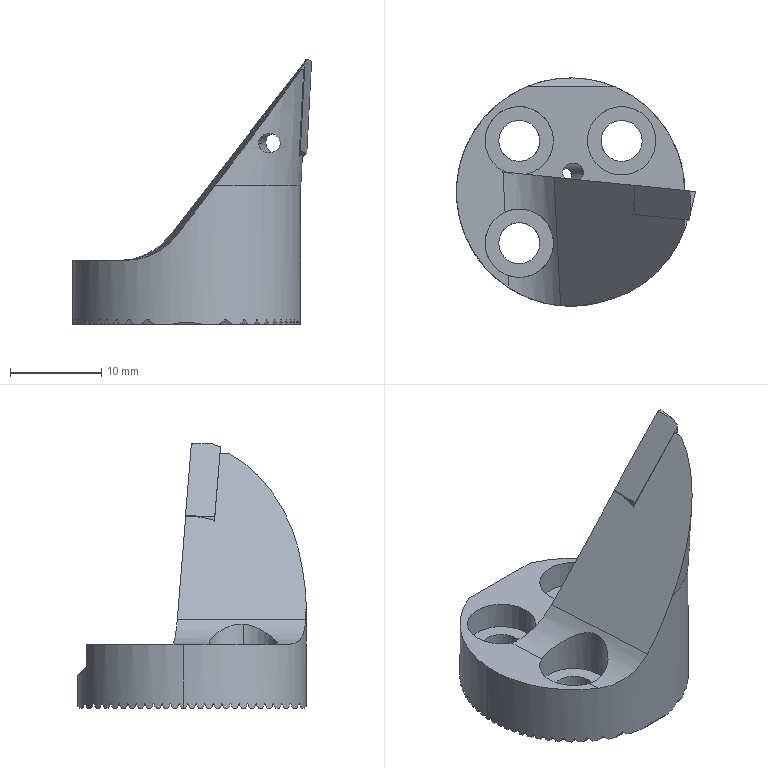NC program | Mastercam | posted with a generic post
Lines 3016 to 4664 of 4664, first 1474 of 1649 lines:
(6 FEM |TOOL - 1|DIA. OFF. - 1|LEN. - 1|TOOL DIA. - 6.)
N6096 T1 M6
N6098 G0 G54 G90 X10.395 Y-5.569 C85.98 B-29.925 S3500 M3
N6100 G43 H1 Z61.524
N6102 Z12.524
N6104 G1 Z11.324 F2000.
N6106 G41 D1 X8.435 Y-5.169 F400.
N6108 X2.979 Y-4.057
N6110 X2.948 Y-4.561
N6112 X8.336 Y-5.659
N6114 G40 X10.295 Y-6.059
N6116 X10.395 Y-5.569
N6118 Z11.124 F2000.
N6120 G41 D1 X8.435 Y-5.169 F400.
N6122 X2.979 Y-4.057
N6124 X2.948 Y-4.561
N6126 X8.336 Y-5.659
N6128 G40 X10.295 Y-6.059
N6130 X10.395 Y-5.569
N6132 Z10.924 F2000.
N6134 G41 D1 X8.435 Y-5.169 F400.
N6136 X2.979 Y-4.057
N6138 X2.948 Y-4.561
N6140 X8.336 Y-5.659
N6142 G40 X10.295 Y-6.059
N6144 X10.395 Y-5.569
N6146 Z10.724 F2000.
N6148 G41 D1 X8.435 Y-5.169 F400.
N6150 X2.979 Y-4.057
N6152 X2.948 Y-4.561
N6154 X8.336 Y-5.659
N6156 G40 X10.295 Y-6.059
N6158 X10.395 Y-5.569
N6160 Z10.524 F2000.
N6162 G41 D1 X8.435 Y-5.169 F400.
N6164 X2.979 Y-4.057
N6166 X2.948 Y-4.561
N6168 X8.336 Y-5.659
N6170 G40 X10.295 Y-6.059
N6172 X10.395 Y-5.569
N6174 Z10.324 F2000.
N6176 G41 D1 X8.435 Y-5.169 F400.
N6178 X2.979 Y-4.057
N6180 X2.948 Y-4.561
N6182 X8.336 Y-5.659
N6184 G40 X10.295 Y-6.059
N6186 X10.395 Y-5.569
N6188 Z10.124 F2000.
N6190 G41 D1 X8.435 Y-5.169 F400.
N6192 X2.979 Y-4.057
N6194 X2.948 Y-4.561
N6196 X8.336 Y-5.659
N6198 G40 X10.295 Y-6.059
N6200 X10.395 Y-5.569
N6202 Z9.924 F2000.
N6204 G41 D1 X8.435 Y-5.169 F400.
N6206 X2.979 Y-4.057
N6208 X2.948 Y-4.561
N6210 X8.336 Y-5.659
N6212 G40 X10.295 Y-6.059
N6214 G0 Z61.524
N6216 M5
N6218 G0 G28 G91 Z0.
N6220 G28 C0. B0.
N6222 M01
N6224 G0 G17 G40 G80 G90 G94 G98
N6226 G0 G28 G91 Z0.
(2 DR |TOOL - 2|DIA. OFF. - 2|LEN. - 2|TOOL DIA. - 2.)
N6228 T2 M6
N6230 G0 G54 G90 X3.096 Y-2.135 C85.98 B-29.925 S150 M3
N6232 G43 H2 Z60.924
N6234 G83 G98 Z2.424 R11.924 Q2. F10.
N6236 G80
N6238 M5
N6240 G0 G28 G91 Z0.
N6242 G28 C0. B0.
N6244 M01
N6246 G0 G17 G40 G80 G90 G94 G98
N6248 G0 G28 G91 Z0.
(12 FEMR |TOOL - 4|DIA. OFF. - 4|LEN. - 4|TOOL DIA. - 12.)
N6250 T4 M6
N6252 G0 G54 G90 X14.729 Y22.915 C6. B-90. S3500 M3
N6254 G43 H4 Z61.514
N6256 Z3.514
N6258 G1 Z1.764 F2000.
N6260 X14.032 Y21.345 Z1.613 F2500.
N6262 G3 X13.8 Y20.25 Z1.514 I2.468 J-1.095
N6264 G1 Y19.651
N6266 Y19.47
N6268 G2 X14.97 Y18.269 I-45.936 J-45.932
N6270 X16.838 Y14.761 I-6.985 J-5.971
N6272 X17.407 Y11.333 I-15.59 J-4.35
N6274 X17.54 Y6.9 I-73.653 J-4.433
N6276 G1 Y6.592
N6278 G2 X17.549 Y2.503 I-899.541 J-4.089
N6280 G1 Y2.175
N6282 Y1.775
N6284 X17.54 Y-12.63
N6286 G2 X16.333 Y-15.954 I-6.352 J.425
N6288 X13.8 Y-18.183 I-6.198 J4.49
N6290 G1 Y-18.582
N6292 Y-18.981
N6294 G3 X16.031 Y-21.64 Z1.764 I2.7
N6296 X16.5 Y-21.681 I.469 J2.659 F9500.
N6298 X19.2 Y-18.981 J2.7
N6300 G1 Y19.725
N6302 G3 X16.5 Y22.425 I-2.7
N6304 X16.031 Y22.384 J-2.7
N6306 X13.8 Y19.725 Z1.514 I.469 J-2.659 F2500.
N6308 G1 Y19.127
N6310 Y18.921
N6312 X14.784 Y17.652
N6314 G2 X16.575 Y13.738 I-9.517 J-6.721
N6316 X17.136 Y10.072 I-19.858 J-4.918
N6318 X17.286 Y5.071 I-83.135 J-5.001
N6320 X17.287 Y4.942 I-83.285
N6322 X17.299 Y.199 I-906.994 J-4.743
N6324 G1 Y-.279
N6326 Y-.679
N6328 X17.297 Y-10.765
N6330 G2 X16.016 Y-14.965 I-7.969 J.136
N6332 X14.326 Y-17.063 I-9.858 J6.212
N6334 G3 X13.905 Y-17.528 I1.14 J-1.455
N6336 X13.8 Y-17.781 I1.048 J-.584
N6338 G1 X14.729 Y-17.96 Z1.576
N6340 G3 X15.651 Y-18.048 Z1.638 I.922 J4.789
N6342 X17.5 Y-17.684 Z1.764 J4.877
N6344 X20.528 Y-13.171 I-1.849 J4.513 F9500.
N6346 X20.516 Y-12.826 I-4.877
N6348 G1 X18.722 Y12.481
N6350 G3 X17.618 Y16.38 I-9.929 J-.704
N6352 G1 X15.156 Y21.1
N6354 X14.729 Y21.919 Z1.702 F2500.
N6356 X14.032 Y20.35 Z1.588
N6358 G3 X13.8 Y19.254 Z1.514 I2.468 J-1.096
N6360 G1 Y18.656
N6362 Y18.445
N6364 X14.667 Y17.103
N6366 G2 X16.375 Y12.756 I-12.15 J-7.284
N6368 X16.922 Y8.354 I-26.107 J-5.48
N6370 X17.043 Y2.631 I-134.973 J-5.723
N6372 G1 X17.042 Y2.11
N6374 G2 X17.047 Y.103 I-910.2 J-3.046
N6376 G1 X17.048 Y-.297
N6378 X17.037 Y-9.694
N6380 G2 X15.43 Y-14.831 I-10.263 J.39
N6382 X14.377 Y-16.348 I-14.569 J8.986
N6384 G1 X14.075 Y-16.691
N6386 G3 X13.8 Y-17.242 I.9 J-.793
N6388 G1 X14.729 Y-17.37 Z1.576
N6390 G3 X15.096 Y-17.395 Z1.6 I.367 J2.675
N6392 X17.232 Y-16.346 Z1.764 J2.7
N6394 X17.791 Y-14.856 I-2.136 J1.651 F9500.
N6396 G1 X19.892 Y20.223
N6398 G3 X19.897 Y20.384 I-2.695 J.161
N6400 X17.197 Y23.084 I-2.7
N6402 X15.24 Y22.245 J-2.7
N6404 X14.729 Y21.48 Z1.702 I1.957 J-1.861 F2500.
N6406 G1 X14.032 Y19.91 Z1.588
N6408 G3 X13.8 Y18.815 Z1.514 I2.468 J-1.095
N6410 G1 Y18.216
N6412 Y17.994
N6414 X14.589 Y16.547
N6416 G2 X16.285 Y11.268 I-15.796 J-7.987
N6418 X16.704 Y6.65 I-36.902 J-5.679
N6420 X16.798 Y-.081 I-239.814 J-6.731
N6422 X16.797 Y-1.122 I-239.908
N6424 G1 Y-1.523
N6426 G2 X16.8 Y-3.681 I-906.97 J-2.158
N6428 X16.787 Y-8.476 I-906.973
N6430 X15.077 Y-14.518 I-12.293 J.216
N6432 X14.239 Y-15.883 I-26.241 J15.167
N6434 G1 X14.033 Y-16.164
N6436 G3 X13.8 Y-16.875 I.967 J-.711
N6438 X16.031 Y-19.534 Z1.764 I2.7
N6440 X16.5 Y-19.575 I.469 J2.659 F9500.
N6442 X19.2 Y-16.875 J2.7
N6444 G1 Y18.386
N6446 G3 X16.5 Y21.086 I-2.7
N6448 X16.031 Y21.045 J-2.7
N6450 X13.8 Y18.386 Z1.514 I.469 J-2.659 F2500.
N6452 G1 Y17.787
N6454 Y17.549
N6456 X14.628 Y15.739
N6458 G2 X16.102 Y10.224 I-19.714 J-8.227
N6460 X16.482 Y4.878 I-48.834 J-6.152
N6462 X16.552 Y-3.377 I-483.428 J-8.255
N6464 X16.549 Y-5.233 I-483.498
N6466 G1 Y-5.633
N6468 G2 X16.552 Y-6.149 I-39.576 J-.516
N6470 X16.488 Y-8.413 I-39.579
N6472 X14.888 Y-14.011 I-14.099 J1.
N6474 X13.984 Y-15.667 I-35.691 J18.427
N6476 G3 X13.8 Y-16.305 I1.016 J-.638
N6478 X16.031 Y-18.964 Z1.764 I2.7
N6480 X16.5 Y-19.005 I.469 J2.659 F9500.
N6482 X19.2 Y-16.305 J2.7
N6484 G1 Y17.963
N6486 G3 X16.5 Y20.663 I-2.7
N6488 X16.031 Y20.622 J-2.7
N6490 X13.8 Y17.963 Z1.514 I.469 J-2.659 F2500.
N6492 G1 Y17.365
N6494 Y17.099
N6496 X14.625 Y14.949
N6498 G2 X15.966 Y8.715 I-24.973 J-8.635
N6500 X16.259 Y2.691 I-71.608 J-6.502
N6502 X16.294 Y-2.883 I-438.719 J-5.574
N6504 X16.277 Y-6.733 I-438.754
N6506 X14.619 Y-13.723 I-16.545 J.233
N6508 G3 X14.142 Y-14.741 I131.524 J-62.248
N6510 G1 X13.926 Y-15.188
N6512 G3 X13.8 Y-15.724 I1.076 J-.536
N6514 G1 Y-16.123
N6516 G3 X16.031 Y-18.782 Z1.764 I2.7
N6518 X16.5 Y-18.823 I.469 J2.659 F9500.
N6520 X19.2 Y-16.123 J2.7
N6522 G1 Y17.537
N6524 G3 X16.5 Y20.237 I-2.7
N6526 X16.031 Y20.196 J-2.7
N6528 X13.8 Y17.537 Z1.514 I.469 J-2.659 F2500.
N6530 G1 Y16.938
N6532 Y16.634
N6534 X14.59 Y14.166
N6536 G2 X15.764 Y7.67 I-30.935 J-8.945
N6538 X16.016 Y1.314 I-88.563 J-6.705
N6540 X16.041 Y-2.954 I-361.608 J-4.268
N6542 X16.032 Y-5.648 I-361.633
N6544 X15.571 Y-9.827 I-20.824 J.181
N6546 X14.278 Y-13.684 I-21.736 J5.14
N6548 G3 X13.888 Y-14.663 I18.448 J-7.926
N6550 X13.8 Y-15.114 I1.112 J-.451
N6552 G1 Y-15.513
N6554 G3 X16.031 Y-18.172 Z1.764 I2.7
N6556 X16.5 Y-18.213 I.469 J2.659 F9500.
N6558 X19.2 Y-15.513 J2.7
N6560 G1 Y17.097
N6562 G3 X16.5 Y19.797 I-2.7
N6564 X16.031 Y19.756 J-2.7
N6566 X13.8 Y17.097 Z1.514 I.469 J-2.659 F2500.
N6568 G1 Y16.499
N6570 G3 X13.789 Y16.322 I1.462 J-.177
N6572 X13.883 Y15.804 I1.473
N6574 X14.089 Y15.056 I143.834 J39.039
N6576 G2 X15.613 Y5.73 I-38.302 J-11.048
N6578 X15.785 Y-1.589 I-155.302 J-7.319
N6580 G1 Y-1.716
N6582 G2 X15.794 Y-2.931 I-85.343 J-1.215
N6584 X15.738 Y-6.002 I-85.352
N6586 X14.402 Y-12.5 I-21.07 J.949
N6588 G3 X13.852 Y-14.096 I31.212 J-11.635
N6590 X13.8 Y-14.447 I1.148 J-.351
N6592 G1 Y-14.846
N6594 G3 X16.031 Y-17.505 Z1.764 I2.7
N6596 X16.5 Y-17.546 I.469 J2.659 F9500.
N6598 X19.2 Y-14.846 J2.7
N6600 G1 Y16.636
N6602 G3 X16.5 Y19.336 I-2.7
N6604 X16.031 Y19.295 J-2.7
N6606 X13.8 Y16.636 Z1.514 I.469 J-2.659 F2500.
N6608 G1 Y16.037
N6610 G3 X13.793 Y15.857 I2.187 J-.18
N6612 X13.856 Y15.332 I2.194
N6614 X14.353 Y13.046 I139.853 J29.205
N6616 G2 X15.389 Y4.704 I-47.631 J-10.149
N6618 X15.527 Y-2.066 I-165.786 J-6.77
N6620 X15.503 Y-4.901 I-165.924
N6622 X14.207 Y-12.123 I-24.214 J.618
N6624 G3 X13.84 Y-13.357 I21.503 J-7.065
N6626 X13.795 Y-13.85 I2.68 J-.493
N6628 X13.8 Y-14.012 I2.725
N6630 G1 Y-14.412
N6632 G3 X16.031 Y-17.071 Z1.764 I2.7
N6634 X16.5 Y-17.112 I.469 J2.659 F9500.
N6636 X19.2 Y-14.412 J2.7
N6638 G1 Y16.154
N6640 G3 X16.5 Y18.854 I-2.7
N6642 X16.031 Y18.813 J-2.7
N6644 X13.8 Y16.154 Z1.514 I.469 J-2.659 F2500.
N6646 G1 Y15.555
N6648 G3 X13.795 Y15.356 I3.962 J-.199
N6650 X13.868 Y14.599 I3.967
N6652 X14.388 Y11.558 I128.842 J20.504
N6654 G2 X15.174 Y3.359 I-59.781 J-9.865
N6656 X15.268 Y-1.868 I-145.694 J-5.227
N6658 X15.25 Y-4.169 I-145.788
N6660 X14.153 Y-11.265 I-27.035 J.544
N6662 G3 X13.833 Y-12.478 I29.887 J-8.55
N6664 X13.791 Y-12.938 I2.486 J-.46
N6666 X13.8 Y-13.156 I2.528
N6668 G1 Y-13.555
N6670 Y-13.988
N6672 Y-13.998
N6674 Y-14.002
N6676 Y-14.212
N6678 Y-14.412
N6680 G3 X16.031 Y-17.071 Z1.764 I2.7
N6682 X16.5 Y-17.112 I.469 J2.659 F9500.
N6684 X19.2 Y-14.412 J2.7
N6686 G1 Y15.656
N6688 G3 X16.5 Y18.356 I-2.7
N6690 X16.031 Y18.315 J-2.7
N6692 X13.8 Y15.656 Z1.514 I.469 J-2.659 F2500.
N6694 G1 Y15.057
N6696 G3 X13.798 Y14.834 I10.86 J-.223
N6698 X13.934 Y13.115 I10.862
N6700 X14.261 Y10.786 I193.248 J25.883
N6702 G2 X14.955 Y1.87 I-75.072 J-10.337
N6704 X15.008 Y-1.441 I-103.205 J-3.311
N6706 X14.975 Y-4.057 I-103.258
N6708 X14.031 Y-10.578 I-30.027 J1.018
N6710 G3 X13.828 Y-11.453 I39.877 J-9.757
N6712 X13.79 Y-11.884 I2.422 J-.431
N6714 X13.8 Y-12.108 I2.46
N6716 G1 Y-12.508
N6718 Y-13.306
N6720 G3 X16.031 Y-15.965 Z1.764 I2.7
N6722 X16.5 Y-16.006 I.469 J2.659 F9500.
N6724 X19.2 Y-13.306 J2.7
N6726 G1 Y15.075
N6728 G3 X16.5 Y17.775 I-2.7
N6730 X16.031 Y17.734 J-2.7
N6732 X13.8 Y15.075 Z1.514 I.469 J-2.659 F2500.
N6734 G1 Y14.476
N6736 Y14.013
N6738 Y14.002
N6740 Y13.998
N6742 G3 X13.799 Y13.81 I17.867 J-.188
N6744 X13.972 Y11.33 I17.868
N6746 X14.105 Y10.152 I402.753 J44.877
N6748 G2 X14.739 Y-.314 I-96.738 J-11.111
N6750 X14.753 Y-1.498 I-50.081 J-1.184
N6752 X14.58 Y-5.654 I-50.095
N6754 X13.851 Y-10.113 I-37.302 J3.806
N6756 G3 X13.791 Y-10.675 I2.591 J-.562
N6758 X13.8 Y-10.891 I2.651
N6760 G1 Y-11.29
N6762 Y-12.088
N6764 G3 X16.031 Y-14.747 Z1.764 I2.7
N6766 X16.5 Y-14.788 I.469 J2.659 F9500.
N6768 X19.2 Y-12.088 J2.7
N6770 G1 Y14.147
N6772 G3 X16.5 Y16.847 I-2.7
N6774 X16.031 Y16.806 J-2.7
N6776 X13.8 Y14.147 Z1.514 I.469 J-2.659 F2500.
N6778 G1 Y14.08
N6780 Y13.998
N6782 Y13.569
N6784 Y13.15
N6786 Y12.751
N6788 G3 X13.797 Y12.368 I26.282 J-.383
N6790 X13.945 Y9.58 I26.285
N6792 X14.013 Y8.79 I806.017 J68.987
N6794 G2 X14.473 Y-1.324 I-110.84 J-10.114
N6796 X14.467 Y-2.527 I-111.3
N6798 X13.817 Y-8.84 I-37.065 J.629
N6800 G3 X13.791 Y-9.22 I2.763 J-.38
N6802 X13.8 Y-9.441 I2.789
N6804 G1 Y-9.84
N6806 Y-11.038
N6808 G3 X16.031 Y-13.697 Z1.764 I2.7
N6810 X16.5 Y-13.738 I.469 J2.659 F9500.
N6812 X19.2 Y-11.038 J2.7
N6814 G1 Y12.551
N6816 G3 X16.5 Y15.251 I-2.7
N6818 X16.031 Y15.21 J-2.7
N6820 X13.8 Y12.551 Z1.514 I.469 J-2.659 F2500.
N6822 G1 Y11.952
N6824 G3 X13.796 Y11.157 I89.637 J-.795
N6826 X13.83 Y8.678 I89.641
N6828 X14.031 Y5.13 I264.013 J13.129
N6830 G2 X14.206 Y-.867 I-102.867 J-5.997
N6832 X14.193 Y-2.466 I-103.042
N6834 X13.81 Y-7.07 I-39.426 J.959
N6836 G3 X13.792 Y-7.411 I3.189 J-.341
N6838 X13.8 Y-7.629 I3.207
N6840 G1 Y-8.028
N6842 Y-9.624
N6844 G3 X16.031 Y-12.283 Z1.764 I2.7
N6846 X16.5 Y-12.324 I.469 J2.659 F9500.
N6848 X19.2 Y-9.624 J2.7
N6850 G1 Y10.282
N6852 G3 X16.5 Y12.982 I-2.7
N6854 X16.031 Y12.941 J-2.7
N6856 X13.8 Y10.282 Z1.514 I.469 J-2.659 F2500.
N6858 G1 Y9.683
N6860 G3 X13.797 Y8.487 I264.088 J-1.196
N6862 X13.819 Y5.062 I264.091
N6864 X13.891 Y2.683 I526.245 J14.664
N6866 G2 X13.946 Y-.182 I-74.989 J-2.865
N6868 X13.88 Y-3.321 I-75.044
N6870 X13.8 Y-4.578 I-41.798 J2.036
N6872 G1 Y-4.977
N6874 Y-7.771
N6876 G3 X16.031 Y-10.43 Z1.764 I2.7
N6878 X16.5 Y-10.471 I.469 J2.659 F9500.
N6880 X19.2 Y-7.771 J2.7
N6882 G1 Y6.753
N6884 G3 X16.5 Y9.453 I-2.7
N6886 X16.031 Y9.412 J-2.7
N6888 X13.8 Y6.753 Z1.514 I.469 J-2.659 F2500.
N6890 G1 Y6.154
N6892 Y-5.021
N6894 G3 X14.032 Y-6.116 Z1.613 I2.7
N6896 G1 X14.729 Y-7.686 Z1.764
N6898 G0 Z61.514
N6900 X13.5 Y22.
N6902 Z52.214
N6904 Z3.214
N6906 G1 Z2.214 F2000.
N6908 G41 D4 Y14. F1000.
N6910 Y-14.
N6912 G40 Y-22.
N6914 G0 Z52.214
N6916 X13.1 Y22.
N6918 Z3.214
N6920 G1 Z2.214 F2000.
N6922 G41 D4 Y14. F1000.
N6924 Y-14.
N6926 G40 Y-22.
N6928 G0 Z52.214
N6930 Z62.563
N6932 X10.617 Y12.777
N6934 C0.
N6936 Z13.563
N6938 G1 Z12.113 F2000.
N6940 G41 D4 Y4.777 F1500.
N6942 Y-4.722
N6944 G40 Y-12.722
N6946 Z11.662 F2000.
N6948 G42 D4 Y-4.722 F1500.
N6950 Y4.777
N6952 G40 Y12.777
N6954 G0 Z62.563
N6956 B-45.
N6958 X-10.997 Y-12.722
N6960 Z62.405
N6962 Z13.405
N6964 G1 Z11.955 F2000.
N6966 G41 D4 Y-4.722 F1500.
N6968 Y4.777
N6970 G40 Y12.777
N6972 Z11.505 F2000.
N6974 G42 D4 Y4.777 F1500.
N6976 Y-4.722
N6978 G40 Y-12.722
N6980 G0 Z62.405
N6982 M5
N6984 G0 G28 G91 Z0.
N6986 G28 B0.
N6988 M01
N6990 G0 G17 G40 G80 G90 G94 G98
N6992 G0 G28 G91 Z0.
(3 FEMR |TOOL - 6|DIA. OFF. - 6|LEN. - 6|TOOL DIA. - 3.)
N6994 T6 M6
N6996 G0 G54 G90 X32.031 Y15.532 C6. B-90. S4500 M3
N6998 G43 H6 Z51.614
N7000 Z2.614
N7002 G1 Z1.422 F2000.
N7004 G41 D6 X31.11 Y15.141 F400.
N7006 X21.543 Y11.08
N7008 X20.313 Y10.119
N7010 X21.734 Y10.193
N7012 X31.173 Y14.2
N7014 G40 X32.094 Y14.591
N7016 X31.445 Y16.913
N7018 G41 D6 X30.524 Y16.522
N7020 X20.775 Y12.384
N7022 X16.033 Y8.679
N7024 X11.648 Y7.04
N7026 G3 X11.55 Y6.899 I.053 J-.141
N7028 X11.701 Y6.748 I.151
N7030 G1 X11.728 Y6.751
N7032 X11.753 Y6.758
N7034 X16.138 Y8.398
N7036 X22.076 Y8.709
N7038 X31.76 Y12.82
N7040 G40 X32.68 Y13.21
N7042 X32.031 Y15.532
N7044 Z1.231 F2000.
N7046 G41 D6 X31.11 Y15.141 F400.
N7048 X21.543 Y11.08
N7050 X20.313 Y10.119
N7052 X21.734 Y10.193
N7054 X31.173 Y14.2
N7056 G40 X32.094 Y14.591
N7058 X31.445 Y16.913
N7060 G41 D6 X30.524 Y16.522
N7062 X20.775 Y12.384
N7064 X16.033 Y8.679
N7066 X11.648 Y7.04
N7068 G3 X11.55 Y6.899 I.053 J-.141
N7070 X11.701 Y6.748 I.151
N7072 G1 X11.728 Y6.751
N7074 X11.753 Y6.758
N7076 X16.138 Y8.398
N7078 X22.076 Y8.709
N7080 X31.76 Y12.82
N7082 G40 X32.68 Y13.21
N7084 X32.031 Y15.532
N7086 Z1.039 F2000.
N7088 G41 D6 X31.11 Y15.141 F400.
N7090 X21.543 Y11.08
N7092 X20.313 Y10.119
N7094 X21.734 Y10.193
N7096 X31.173 Y14.2
N7098 G40 X32.094 Y14.591
N7100 X31.445 Y16.913
N7102 G41 D6 X30.524 Y16.522
N7104 X20.775 Y12.384
N7106 X16.033 Y8.679
N7108 X11.648 Y7.04
N7110 G3 X11.55 Y6.899 I.053 J-.141
N7112 X11.701 Y6.748 I.151
N7114 G1 X11.728 Y6.751
N7116 X11.753 Y6.758
N7118 X16.138 Y8.398
N7120 X22.076 Y8.709
N7122 X31.76 Y12.82
N7124 G40 X32.68 Y13.21
N7126 X32.031 Y15.532
N7128 Z.848 F2000.
N7130 G41 D6 X31.11 Y15.141 F400.
N7132 X21.543 Y11.08
N7134 X20.313 Y10.119
N7136 X21.734 Y10.193
N7138 X31.173 Y14.2
N7140 G40 X32.094 Y14.591
N7142 X31.445 Y16.913
N7144 G41 D6 X30.524 Y16.522
N7146 X20.775 Y12.384
N7148 X16.033 Y8.679
N7150 X11.648 Y7.04
N7152 G3 X11.55 Y6.899 I.053 J-.141
N7154 X11.701 Y6.748 I.151
N7156 G1 X11.728 Y6.751
N7158 X11.753 Y6.758
N7160 X16.138 Y8.398
N7162 X22.076 Y8.709
N7164 X31.76 Y12.82
N7166 G40 X32.68 Y13.21
N7168 X32.031 Y15.532
N7170 Z.656 F2000.
N7172 G41 D6 X31.11 Y15.141 F400.
N7174 X21.543 Y11.08
N7176 X20.313 Y10.119
N7178 X21.734 Y10.193
N7180 X31.173 Y14.2
N7182 G40 X32.094 Y14.591
N7184 X31.445 Y16.913
N7186 G41 D6 X30.524 Y16.522
N7188 X20.775 Y12.384
N7190 X16.033 Y8.679
N7192 X11.648 Y7.04
N7194 G3 X11.55 Y6.899 I.053 J-.141
N7196 X11.701 Y6.748 I.151
N7198 G1 X11.728 Y6.751
N7200 X11.753 Y6.758
N7202 X16.138 Y8.398
N7204 X22.076 Y8.709
N7206 X31.76 Y12.82
N7208 G40 X32.68 Y13.21
N7210 X32.031 Y15.532
N7212 Z.465 F2000.
N7214 G41 D6 X31.11 Y15.141 F400.
N7216 X21.543 Y11.08
N7218 X20.313 Y10.119
N7220 X21.734 Y10.193
N7222 X31.173 Y14.2
N7224 G40 X32.094 Y14.591
N7226 X31.445 Y16.913
N7228 G41 D6 X30.524 Y16.522
N7230 X20.775 Y12.384
N7232 X16.033 Y8.679
N7234 X11.648 Y7.04
N7236 G3 X11.55 Y6.899 I.053 J-.141
N7238 X11.701 Y6.748 I.151
N7240 G1 X11.728 Y6.751
N7242 X11.753 Y6.758
N7244 X16.138 Y8.398
N7246 X22.076 Y8.709
N7248 X31.76 Y12.82
N7250 G40 X32.68 Y13.21
N7252 X32.031 Y15.532
N7254 Z.273 F2000.
N7256 G41 D6 X31.11 Y15.141 F400.
N7258 X21.543 Y11.08
N7260 X20.313 Y10.119
N7262 X21.734 Y10.193
N7264 X31.173 Y14.2
N7266 G40 X32.094 Y14.591
N7268 X31.445 Y16.913
N7270 G41 D6 X30.524 Y16.522
N7272 X20.775 Y12.384
N7274 X16.033 Y8.679
N7276 X11.648 Y7.04
N7278 G3 X11.55 Y6.899 I.053 J-.141
N7280 X11.701 Y6.748 I.151
N7282 G1 X11.728 Y6.751
N7284 X11.753 Y6.758
N7286 X16.138 Y8.398
N7288 X22.076 Y8.709
N7290 X31.76 Y12.82
N7292 G40 X32.68 Y13.21
N7294 X32.031 Y15.532
N7296 Z.082 F2000.
N7298 G41 D6 X31.11 Y15.141 F400.
N7300 X21.543 Y11.08
N7302 X20.313 Y10.119
N7304 X21.734 Y10.193
N7306 X31.173 Y14.2
N7308 G40 X32.094 Y14.591
N7310 X31.445 Y16.913
N7312 G41 D6 X30.524 Y16.522
N7314 X20.775 Y12.384
N7316 X16.033 Y8.679
N7318 X11.648 Y7.04
N7320 G3 X11.55 Y6.899 I.053 J-.141
N7322 X11.701 Y6.748 I.151
N7324 G1 X11.728 Y6.751
N7326 X11.753 Y6.758
N7328 X16.138 Y8.398
N7330 X22.076 Y8.709
N7332 X31.76 Y12.82
N7334 G40 X32.68 Y13.21
N7336 X32.031 Y15.532
N7338 Z-.11 F2000.
N7340 G41 D6 X31.11 Y15.141 F400.
N7342 X21.543 Y11.08
N7344 X20.313 Y10.119
N7346 X21.734 Y10.193
N7348 X31.173 Y14.2
N7350 G40 X32.094 Y14.591
N7352 X31.445 Y16.913
N7354 G41 D6 X30.524 Y16.522
N7356 X20.775 Y12.384
N7358 X16.033 Y8.679
N7360 X11.648 Y7.04
N7362 G3 X11.55 Y6.899 I.053 J-.141
N7364 X11.701 Y6.748 I.151
N7366 G1 X11.728 Y6.751
N7368 X11.753 Y6.758
N7370 X16.138 Y8.398
N7372 X22.076 Y8.709
N7374 X31.76 Y12.82
N7376 G40 X32.68 Y13.21
N7378 X32.031 Y15.532
N7380 Z-.301 F2000.
N7382 G41 D6 X31.11 Y15.141 F400.
N7384 X21.543 Y11.08
N7386 X20.313 Y10.119
N7388 X21.734 Y10.193
N7390 X31.173 Y14.2
N7392 G40 X32.094 Y14.591
N7394 X31.445 Y16.913
N7396 G41 D6 X30.524 Y16.522
N7398 X20.775 Y12.384
N7400 X16.033 Y8.679
N7402 X11.648 Y7.04
N7404 G3 X11.55 Y6.899 I.053 J-.141
N7406 X11.701 Y6.748 I.151
N7408 G1 X11.728 Y6.751
N7410 X11.753 Y6.758
N7412 X16.138 Y8.398
N7414 X22.076 Y8.709
N7416 X31.76 Y12.82
N7418 G40 X32.68 Y13.21
N7420 X32.031 Y15.532
N7422 Z-.492 F2000.
N7424 G41 D6 X31.11 Y15.141 F400.
N7426 X21.543 Y11.08
N7428 X20.313 Y10.119
N7430 X21.734 Y10.193
N7432 X31.173 Y14.2
N7434 G40 X32.094 Y14.591
N7436 X31.445 Y16.913
N7438 G41 D6 X30.524 Y16.522
N7440 X20.775 Y12.384
N7442 X16.033 Y8.679
N7444 X11.648 Y7.04
N7446 G3 X11.55 Y6.899 I.053 J-.141
N7448 X11.701 Y6.748 I.151
N7450 G1 X11.728 Y6.751
N7452 X11.753 Y6.758
N7454 X16.138 Y8.398
N7456 X22.076 Y8.709
N7458 X31.76 Y12.82
N7460 G40 X32.68 Y13.21
N7462 X32.031 Y15.532
N7464 Z-.684 F2000.
N7466 G41 D6 X31.11 Y15.141 F400.
N7468 X21.543 Y11.08
N7470 X20.313 Y10.119
N7472 X21.734 Y10.193
N7474 X31.173 Y14.2
N7476 G40 X32.094 Y14.591
N7478 X31.445 Y16.913
N7480 G41 D6 X30.524 Y16.522
N7482 X20.775 Y12.384
N7484 X16.033 Y8.679
N7486 X11.648 Y7.04
N7488 G3 X11.55 Y6.899 I.053 J-.141
N7490 X11.701 Y6.748 I.151
N7492 G1 X11.728 Y6.751
N7494 X11.753 Y6.758
N7496 X16.138 Y8.398
N7498 X22.076 Y8.709
N7500 X31.76 Y12.82
N7502 G40 X32.68 Y13.21
N7504 X32.031 Y15.532
N7506 Z-.875 F2000.
N7508 G41 D6 X31.11 Y15.141 F400.
N7510 X21.543 Y11.08
N7512 X20.313 Y10.119
N7514 X21.734 Y10.193
N7516 X31.173 Y14.2
N7518 G40 X32.094 Y14.591
N7520 X31.445 Y16.913
N7522 G41 D6 X30.524 Y16.522
N7524 X20.775 Y12.384
N7526 X16.033 Y8.679
N7528 X11.648 Y7.04
N7530 G3 X11.55 Y6.899 I.053 J-.141
N7532 X11.701 Y6.748 I.151
N7534 G1 X11.728 Y6.751
N7536 X11.753 Y6.758
N7538 X16.138 Y8.398
N7540 X22.076 Y8.709
N7542 X31.76 Y12.82
N7544 G40 X32.68 Y13.21
N7546 X32.031 Y15.532
N7548 Z-1.067 F2000.
N7550 G41 D6 X31.11 Y15.141 F400.
N7552 X21.543 Y11.08
N7554 X20.313 Y10.119
N7556 X21.734 Y10.193
N7558 X31.173 Y14.2
N7560 G40 X32.094 Y14.591
N7562 X31.445 Y16.913
N7564 G41 D6 X30.524 Y16.522
N7566 X20.775 Y12.384
N7568 X16.033 Y8.679
N7570 X11.648 Y7.04
N7572 G3 X11.55 Y6.899 I.053 J-.141
N7574 X11.701 Y6.748 I.151
N7576 G1 X11.728 Y6.751
N7578 X11.753 Y6.758
N7580 X16.138 Y8.398
N7582 X22.076 Y8.709
N7584 X31.76 Y12.82
N7586 G40 X32.68 Y13.21
N7588 X32.031 Y15.532
N7590 Z-1.258 F2000.
N7592 G41 D6 X31.11 Y15.141 F400.
N7594 X21.543 Y11.08
N7596 X20.313 Y10.119
N7598 X21.734 Y10.193
N7600 X31.173 Y14.2
N7602 G40 X32.094 Y14.591
N7604 X31.445 Y16.913
N7606 G41 D6 X30.524 Y16.522
N7608 X20.775 Y12.384
N7610 X16.033 Y8.679
N7612 X11.648 Y7.04
N7614 G3 X11.55 Y6.899 I.053 J-.141
N7616 X11.701 Y6.748 I.151
N7618 G1 X11.728 Y6.751
N7620 X11.753 Y6.758
N7622 X16.138 Y8.398
N7624 X22.076 Y8.709
N7626 X31.76 Y12.82
N7628 G40 X32.68 Y13.21
N7630 X32.031 Y15.532
N7632 Z-1.45 F2000.
N7634 G41 D6 X31.11 Y15.141 F400.
N7636 X21.543 Y11.08
N7638 X20.313 Y10.119
N7640 X21.734 Y10.193
N7642 X31.173 Y14.2
N7644 G40 X32.094 Y14.591
N7646 X31.445 Y16.913
N7648 G41 D6 X30.524 Y16.522
N7650 X20.775 Y12.384
N7652 X16.033 Y8.679
N7654 X11.648 Y7.04
N7656 G3 X11.55 Y6.899 I.053 J-.141
N7658 X11.701 Y6.748 I.151
N7660 G1 X11.728 Y6.751
N7662 X11.753 Y6.758
N7664 X16.138 Y8.398
N7666 X22.076 Y8.709
N7668 X31.76 Y12.82
N7670 G40 X32.68 Y13.21
N7672 X32.031 Y15.532
N7674 Z-1.641 F2000.
N7676 G41 D6 X31.11 Y15.141 F400.
N7678 X21.543 Y11.08
N7680 X20.313 Y10.119
N7682 X21.734 Y10.193
N7684 X31.173 Y14.2
N7686 G40 X32.094 Y14.591
N7688 X31.445 Y16.913
N7690 G41 D6 X30.524 Y16.522
N7692 X20.775 Y12.384
N7694 X16.033 Y8.679
N7696 X11.648 Y7.04
N7698 G3 X11.55 Y6.899 I.053 J-.141
N7700 X11.701 Y6.748 I.151
N7702 G1 X11.728 Y6.751
N7704 X11.753 Y6.758
N7706 X16.138 Y8.398
N7708 X22.076 Y8.709
N7710 X31.76 Y12.82
N7712 G40 X32.68 Y13.21
N7714 G0 Z51.614
N7716 M5
N7718 G0 G28 G91 Z0.
N7720 G28 C0. B0.
N7722 M01
N7724 G0 G17 G40 G80 G90 G94 G98
N7726 G0 G28 G91 Z0.
(3 FEMF |TOOL - 7|DIA. OFF. - 7|LEN. - 7|TOOL DIA. - 3.)
N7728 T7 M6
N7730 G0 G54 G90 X31.624 Y15.468 C6. B-90. S4500 M3
N7732 G43 H7 Z48.269
N7734 Z-.731
N7736 G1 Z-1.731 F2000.
N7738 G41 D7 X31.071 Y15.233 F400.
N7740 X21.492 Y11.167
N7742 X20.001 Y10.003
N7744 X21.757 Y10.095
N7746 X31.213 Y14.108
N7748 G40 X31.765 Y14.343
N7750 X31.037 Y16.849
N7752 G41 D7 X30.485 Y16.614
N7754 X20.724 Y12.471
N7756 X15.984 Y8.767
N7758 X11.613 Y7.133
N7760 G3 X11.451 Y6.899 I.088 J-.234
N7762 X11.701 Y6.649 I.25
N7764 X11.789 Y6.665 J.25
N7766 G1 X16.159 Y8.299
N7768 X22.099 Y8.61
N7770 X31.799 Y12.728
N7772 G40 X32.351 Y12.962
N7774 G0 Z48.269
N7776 X31.624 Y15.468 Z48.259
N7778 Z-.741
N7780 G1 Z-1.741 F2000.
N7782 G41 D7 X31.071 Y15.233 F400.
N7784 X21.492 Y11.167
N7786 X20.001 Y10.003
N7788 X21.757 Y10.095
N7790 X31.213 Y14.108
N7792 G40 X31.765 Y14.343
N7794 X31.037 Y16.849
N7796 G41 D7 X30.485 Y16.614
N7798 X20.724 Y12.471
N7800 X15.984 Y8.767
N7802 X11.613 Y7.133
N7804 G3 X11.451 Y6.899 I.088 J-.234
N7806 X11.701 Y6.649 I.25
N7808 X11.789 Y6.665 J.25
N7810 G1 X16.159 Y8.299
N7812 X22.099 Y8.61
N7814 X31.799 Y12.728
N7816 G40 X32.351 Y12.962
N7818 G0 Z48.259
N7820 M5
N7822 G0 G28 G91 Z0.
N7824 G28 C0. B0.
N7826 M01
N7828 G0 G17 G40 G80 G90 G94 G98
N7830 G0 G28 G91 Z0.
(2X7 DCHC |TOOL - 8|DIA. OFF. - 8|LEN. - 8|TOOL DIA. - 6.)
N7832 T8 M6
N7834 G0 G54 G90 X20.345 Y12.4 C6. B-90. S3500 M3
N7836 G43 H8 Z49.863
N7838 Z.863
N7840 G1 Z-1.137 F2000.
N7842 G41 D8 X19.399 Y11.661 F400.
N7844 X14.777 Y8.049
N7846 X20.881 Y8.369
N7848 G40 X22.08 Y8.432
N7850 X20.283 Y12.478
N7852 G41 D8 X19.338 Y11.74
N7854 X14.465 Y7.933
N7856 X20.886 Y8.269
N7858 G40 X22.085 Y8.332
N7860 X20.222 Y12.557
N7862 G41 D8 X19.276 Y11.818
N7864 X14.154 Y7.816
N7866 X20.892 Y8.169
N7868 G40 X22.09 Y8.232
N7870 X20.222 Y12.557
N7872 G41 D8 X19.276 Y11.818
N7874 X14.154 Y7.816
N7876 X20.892 Y8.169
N7878 G40 X22.09 Y8.232
N7880 G0 Z49.863
N7882 M5
N7884 G0 G28 G91 Z0.
N7886 G28 C0. B0.
N7888 M01
N7890 G0 G17 G40 G80 G90 G94 G98
N7892 G0 G28 G91 Z0.
(12 FEMF |TOOL - 9|DIA. OFF. - 9|LEN. - 9|TOOL DIA. - 12.)
N7894 T9 M6
N7896 G0 G54 G90 X13. Y16.006 C177. B-90. S3500 M3
N7898 G43 H9 Z47.418
N7900 Z-1.582
N7902 G1 Z-4.582 F2000.
N7904 G41 D9 Y13.606 F600.
N7906 Y7.266
N7908 G3 X13.389 Y6.474 I1.
N7910 G1 X31.527 Y-7.523
N7912 G2 X33.939 Y-12.431 I-3.788 J-4.908
N7914 X27.739 Y-18.631 I-6.2
N7916 X27.418 Y-18.623 J6.2
N7918 G1 X27.407
N7920 G3 X27.208 Y-18.812 J-.2
N7922 G1 G40 X27.083 Y-21.209
N7924 G0 Z47.418
N7926 Z52.214
N7928 X-13. Y-22.
N7930 C186. B-270.
N7932 Z3.214
N7934 G1 Z2.214 F2000.
N7936 G41 D9 Y-14. F600.
N7938 Y14.
N7940 G40 Y22.
N7942 G0 Z52.214
N7944 Z61.563
N7946 X-10.517 Y-12.777
N7948 C180.
N7950 Z12.563
N7952 G1 Z11.563 F2000.
N7954 G41 D9 Y-4.777 F600.
N7956 Y4.722
N7958 G40 Y12.722
N7960 G0 Z61.563
N7962 B-315.
N7964 X10.897
N7966 Z61.405
N7968 Z12.405
N7970 G1 Z11.405 F2000.
N7972 G41 D9 Y4.722 F600.
N7974 Y-4.777
N7976 G40 Y-12.777
N7978 G0 Z61.405
N7980 M5
N7982 G0 G28 G91 Z0.
N7984 G28 C0. B0.
N7986 M01
N7988 G0 G17 G40 G80 G90 G94 G98
N7990 G0 G28 G91 Z0.
(30 BNOS |TOOL - 10|DIA. OFF. - 10|LEN. - 10|TOOL DIA. - 30.)
N7992 T10 M6
N7994 G0 G54 G90 X22. Y32. C6. B-90. S3000 M3
N7996 G43 H10 Z51.414
N7998 Z2.414
N8000 G1 Z1.414 F2000.
N8002 G41 D10 Y14. F400.
N8004 Y-14.
N8006 G40 Y-32.
N8008 G0 Z51.414
N8010 M5
N8012 G0 G28 G91 Z0.
N8014 G28 C0. B0.
N8016 M01
N8018 G0 G17 G40 G80 G90 G94 G98
N8020 G0 G28 G91 Z0.
(5 SPD |TOOL - 12|DIA. OFF. - 12|LEN. - 12|TOOL DIA. - 5.)
N8022 T12 M6
N8024 G0 G54 G90 X19.859 Y9.95 C6. B-90. S2000 M3
N8026 G43 H12 Z48.259
N8028 G81 G98 Z-3.141 R-.741 F100.
N8030 G80
N8032 M5
N8034 G0 G28 G91 Z0.
N8036 G28 C0. B0.
N8038 M01
N8040 G0 G17 G40 G80 G90 G94 G98
N8042 G0 G28 G91 Z0.
(2.1 DR |TOOL - 13|DIA. OFF. - 13|LEN. - 13|TOOL DIA. - 2.1)
N8044 T13 M6
N8046 G0 G54 G90 X19.859 Y9.95 C6. B-90. S2500 M3
N8048 G43 H13 Z48.259
N8050 G83 G98 Z-9.741 R-.741 Q2. F40.
N8052 G80
N8054 M5
N8056 G0 G28 G91 Z0.
N8058 G28 C0. B0.
N8060 M01
N8062 G0 G17 G40 G80 G90 G94 G98
N8064 G0 G28 G91 Z0.
(2.5 FEM |TOOL - 11|DIA. OFF. - 11|LEN. - 11|TOOL DIA. - 2.5)
N8066 T11 M6
N8068 G0 G54 G90 X19.859 Y-9.95 C186. B-90. S4000 M3
N8070 G43 H11 Z59.147
N8072 G83 G98 Z6.347 R10.147 Q1. F40.
N8074 G80
N8076 M5
N8078 G0 G28 G91 Z0.
N8080 G28 C0. B0.
N8082 M01
N8084 G0 G17 G40 G80 G90 G94 G98
N8086 G0 G28 G91 Z0.
(1.95 THML |TOOL - 14|DIA. OFF. - 14|LEN. - 14|TOOL DIA. - 1.95)
N8088 T14 M6
N8090 G0 G54 G90 X19.859 Y-9.95 C186. B-90. S3000 M3
N8092 G43 H14 Z51.741
N8094 Z3.741
N8096 G1 Z1.291 F2000.
N8098 G41 D14 X19.984 F200.
N8100 G3 X19.859 Y-9.825 Z1.404 I-.125
N8102 X19.734 Y-9.95 Z1.516 J-.125
N8104 X19.859 Y-10.075 Z1.629 I.125
N8106 X19.984 Y-9.95 Z1.742 J.125
N8108 X19.859 Y-9.825 Z1.854 I-.125
N8110 X19.734 Y-9.95 Z1.966 J-.125
N8112 G1 G40 X19.859
N8114 Z2.641 F2000.
N8116 G41 D14 X19.984 F200.
N8118 G3 X19.859 Y-9.825 Z2.754 I-.125
N8120 X19.734 Y-9.95 Z2.866 J-.125
N8122 X19.859 Y-10.075 Z2.979 I.125
N8124 X19.984 Y-9.95 Z3.091 J.125
N8126 X19.859 Y-9.825 Z3.204 I-.125
N8128 X19.734 Y-9.95 Z3.316 J-.125
N8130 G1 G40 X19.859
N8132 G0 Z3.991
N8134 G1 G41 D14 X19.984
N8136 G3 X19.859 Y-9.825 Z4.104 I-.125
N8138 X19.734 Y-9.95 Z4.216 J-.125
N8140 X19.859 Y-10.075 Z4.329 I.125
N8142 X19.984 Y-9.95 Z4.441 J.125
N8144 X19.859 Y-9.825 Z4.554 I-.125
N8146 X19.734 Y-9.95 Z4.666 J-.125
N8148 G1 G40 X19.859
N8150 G0 Z5.341
N8152 G1 G41 D14 X19.984
N8154 G3 X19.859 Y-9.825 Z5.454 I-.125
N8156 X19.734 Y-9.95 Z5.566 J-.125
N8158 X19.859 Y-10.075 Z5.679 I.125
N8160 X19.984 Y-9.95 Z5.792 J.125
N8162 X19.859 Y-9.825 Z5.904 I-.125
N8164 X19.734 Y-9.95 Z6.016 J-.125
N8166 G1 G40 X19.859
N8168 Z1.291 F2000.
N8170 G41 D14 X20.034 F200.
N8172 G3 X19.859 Y-9.775 Z1.404 I-.175
N8174 X19.684 Y-9.95 Z1.516 J-.175
N8176 X19.859 Y-10.125 Z1.629 I.175
N8178 X20.034 Y-9.95 Z1.742 J.175
N8180 X19.859 Y-9.775 Z1.854 I-.175
N8182 X19.684 Y-9.95 Z1.966 J-.175
N8184 G1 G40 X19.859
N8186 Z2.641 F2000.
N8188 G41 D14 X20.034 F200.
N8190 G3 X19.859 Y-9.775 Z2.754 I-.175
N8192 X19.684 Y-9.95 Z2.866 J-.175
N8194 X19.859 Y-10.125 Z2.979 I.175
N8196 X20.034 Y-9.95 Z3.091 J.175
N8198 X19.859 Y-9.775 Z3.204 I-.175
N8200 X19.684 Y-9.95 Z3.316 J-.175
N8202 G1 G40 X19.859
N8204 G0 Z3.991
N8206 G1 G41 D14 X20.034
N8208 G3 X19.859 Y-9.775 Z4.104 I-.175
N8210 X19.684 Y-9.95 Z4.216 J-.175
N8212 X19.859 Y-10.125 Z4.329 I.175
N8214 X20.034 Y-9.95 Z4.441 J.175
N8216 X19.859 Y-9.775 Z4.554 I-.175
N8218 X19.684 Y-9.95 Z4.666 J-.175
N8220 G1 G40 X19.859
N8222 G0 Z5.341
N8224 G1 G41 D14 X20.034
N8226 G3 X19.859 Y-9.775 Z5.454 I-.175
N8228 X19.684 Y-9.95 Z5.566 J-.175
N8230 X19.859 Y-10.125 Z5.679 I.175
N8232 X20.034 Y-9.95 Z5.792 J.175
N8234 X19.859 Y-9.775 Z5.904 I-.175
N8236 X19.684 Y-9.95 Z6.016 J-.175
N8238 G1 G40 X19.859
N8240 Z1.291 F2000.
N8242 G41 D14 X20.084 F200.
N8244 G3 X19.859 Y-9.725 Z1.404 I-.225
N8246 X19.634 Y-9.95 Z1.516 J-.225
N8248 X19.859 Y-10.175 Z1.629 I.225
N8250 X20.084 Y-9.95 Z1.742 J.225
N8252 X19.859 Y-9.725 Z1.854 I-.225
N8254 X19.634 Y-9.95 Z1.966 J-.225
N8256 G1 G40 X19.859
N8258 Z2.641 F2000.
N8260 G41 D14 X20.084 F200.
N8262 G3 X19.859 Y-9.725 Z2.754 I-.225
N8264 X19.634 Y-9.95 Z2.866 J-.225
N8266 X19.859 Y-10.175 Z2.979 I.225
N8268 X20.084 Y-9.95 Z3.091 J.225
N8270 X19.859 Y-9.725 Z3.204 I-.225
N8272 X19.634 Y-9.95 Z3.316 J-.225
N8274 G1 G40 X19.859
N8276 G0 Z3.991
N8278 G1 G41 D14 X20.084
N8280 G3 X19.859 Y-9.725 Z4.104 I-.225
N8282 X19.634 Y-9.95 Z4.216 J-.225
N8284 X19.859 Y-10.175 Z4.329 I.225
N8286 X20.084 Y-9.95 Z4.441 J.225
N8288 X19.859 Y-9.725 Z4.554 I-.225
N8290 X19.634 Y-9.95 Z4.666 J-.225
N8292 G1 G40 X19.859
N8294 G0 Z5.341
N8296 G1 G41 D14 X20.084
N8298 G3 X19.859 Y-9.725 Z5.454 I-.225
N8300 X19.634 Y-9.95 Z5.566 J-.225
N8302 X19.859 Y-10.175 Z5.679 I.225
N8304 X20.084 Y-9.95 Z5.792 J.225
N8306 X19.859 Y-9.725 Z5.904 I-.225
N8308 X19.634 Y-9.95 Z6.016 J-.225
N8310 G1 G40 X19.859
N8312 Z1.291 F2000.
N8314 G41 D14 X20.134 F200.
N8316 G3 X19.859 Y-9.675 Z1.404 I-.275
N8318 X19.584 Y-9.95 Z1.516 J-.275
N8320 X19.859 Y-10.225 Z1.629 I.275
N8322 X20.134 Y-9.95 Z1.742 J.275
N8324 X19.859 Y-9.675 Z1.854 I-.275
N8326 X19.584 Y-9.95 Z1.966 J-.275
N8328 G1 G40 X19.859
N8330 Z2.641 F2000.
N8332 G41 D14 X20.134 F200.
N8334 G3 X19.859 Y-9.675 Z2.754 I-.275
N8336 X19.584 Y-9.95 Z2.866 J-.275
N8338 X19.859 Y-10.225 Z2.979 I.275
N8340 X20.134 Y-9.95 Z3.091 J.275
N8342 X19.859 Y-9.675 Z3.204 I-.275
N8344 X19.584 Y-9.95 Z3.316 J-.275
N8346 G1 G40 X19.859
N8348 G0 Z3.991
N8350 G1 G41 D14 X20.134
N8352 G3 X19.859 Y-9.675 Z4.104 I-.275
N8354 X19.584 Y-9.95 Z4.216 J-.275
N8356 X19.859 Y-10.225 Z4.329 I.275
N8358 X20.134 Y-9.95 Z4.441 J.275
N8360 X19.859 Y-9.675 Z4.554 I-.275
N8362 X19.584 Y-9.95 Z4.666 J-.275
N8364 G1 G40 X19.859
N8366 G0 Z5.341
N8368 G1 G41 D14 X20.134
N8370 G3 X19.859 Y-9.675 Z5.454 I-.275
N8372 X19.584 Y-9.95 Z5.566 J-.275
N8374 X19.859 Y-10.225 Z5.679 I.275
N8376 X20.134 Y-9.95 Z5.792 J.275
N8378 X19.859 Y-9.675 Z5.904 I-.275
N8380 X19.584 Y-9.95 Z6.016 J-.275
N8382 G1 G40 X19.859
N8384 Z1.291 F2000.
N8386 G41 D14 X20.134 F200.
N8388 G3 X19.859 Y-9.675 Z1.404 I-.275
N8390 X19.584 Y-9.95 Z1.516 J-.275
N8392 X19.859 Y-10.225 Z1.629 I.275
N8394 X20.134 Y-9.95 Z1.742 J.275
N8396 X19.859 Y-9.675 Z1.854 I-.275
N8398 X19.584 Y-9.95 Z1.966 J-.275
N8400 G1 G40 X19.859
N8402 Z2.641 F2000.
N8404 G41 D14 X20.134 F200.
N8406 G3 X19.859 Y-9.675 Z2.754 I-.275
N8408 X19.584 Y-9.95 Z2.866 J-.275
N8410 X19.859 Y-10.225 Z2.979 I.275
N8412 X20.134 Y-9.95 Z3.091 J.275
N8414 X19.859 Y-9.675 Z3.204 I-.275
N8416 X19.584 Y-9.95 Z3.316 J-.275
N8418 G1 G40 X19.859
N8420 G0 Z3.991
N8422 G1 G41 D14 X20.134
N8424 G3 X19.859 Y-9.675 Z4.104 I-.275
N8426 X19.584 Y-9.95 Z4.216 J-.275
N8428 X19.859 Y-10.225 Z4.329 I.275
N8430 X20.134 Y-9.95 Z4.441 J.275
N8432 X19.859 Y-9.675 Z4.554 I-.275
N8434 X19.584 Y-9.95 Z4.666 J-.275
N8436 G1 G40 X19.859
N8438 G0 Z5.341
N8440 G1 G41 D14 X20.134
N8442 G3 X19.859 Y-9.675 Z5.454 I-.275
N8444 X19.584 Y-9.95 Z5.566 J-.275
N8446 X19.859 Y-10.225 Z5.679 I.275
N8448 X20.134 Y-9.95 Z5.792 J.275
N8450 X19.859 Y-9.675 Z5.904 I-.275
N8452 X19.584 Y-9.95 Z6.016 J-.275
N8454 G1 G40 X19.859
N8456 G0 Z51.741
N8458 M5
N8460 G0 G28 G91 Z0.
N8462 G28 C0. B0.
N8464 M01
N8466 G0 G17 G40 G80 G90 G94 G98
N8468 G0 G28 G91 Z0.
(2.5 BM |TOOL - 15|DIA. OFF. - 15|LEN. - 15|TOOL DIA. - 2.5)
N8470 T15 M6
N8472 G0 G54 G90 X18.575 Y13.252 C48.214 B-90. S5000 M3
N8474 G43 H15 Z48.212
N8476 Y8.411
N8478 Z30.603
N8480 Z12.603
N8482 G1 Z10.603 F2000.
N8484 X18.593 Z9.77 F1000.
N8486 X18.582 Z9.697
N8488 X18.548 Y8.409 Z9.631
N8490 X18.495 Y8.406 Z9.573
N8492 X18.427 Y8.402 Z9.522
N8494 X18.267 Y8.393 Z9.448
N8496 X18.106 Y8.384 Z9.419
N8498 X17.861 Y8.34 Z9.437 C48.401
N8500 X17.372 Y8.251 Z9.474 C48.773
N8502 X16.883 Y8.162 Z9.51 C49.146
N8504 X16.395 Y8.073 Z9.545 C49.52
N8506 X15.906 Y7.985 Z9.58 C49.893
N8508 X15.437 Y7.897 Z9.612 C50.244
N8510 X14.968 Y7.819 Z9.651 C50.595
N8512 X14.479 Y7.751 Z9.699 C50.95
N8514 X13.989 Y7.686 Z9.745 C51.291
N8516 X13.499 Y7.62 Z9.791 C51.632
N8518 X13.01 Y7.561 Z9.831 C51.94
N8520 X12.52 Y7.501 Z9.872 C52.248
N8522 X12.031 Y7.441 Z9.912 C52.556
N8524 X11.541 Y7.381 Z9.952 C52.864
N8526 X11.052 Y7.337 Z9.981 C53.088
N8528 X10.562 Y7.293 Z10.009 C53.311
N8530 X10.072 Y7.249 Z10.038 C53.535
N8532 X9.583 Y7.205 Z10.066 C53.759
N8534 X9.093 Y7.185 Z10.078 C53.859
N8536 X8.604 Y7.165 Z10.091 C53.959
N8538 X8.114 Y7.146 Z10.103 C54.059
N8540 X8.043 Y7.141 Z10.109 C54.069
N8542 X7.972 Y7.135 Z10.115 C54.079
N8544 X7.901 Y7.13 Z10.121 C54.089
N8546 X7.83 Y7.128 Z10.126 C54.085
N8548 X7.827 Y7.124 C54.084
N8550 X7.824 Y7.12
N8552 X7.821 Y7.116 Z10.125
N8554 X7.817 Y7.112 C54.083
N8556 X7.814 Y7.108
N8558 X7.811 Y7.104
N8560 X7.807 Y7.1 C54.082
N8562 X7.804 Y7.096
N8564 X7.805 Y7.08 Z10.127 C54.081
N8566 X7.806 Y7.064 Z10.129 C54.08
N8568 X7.807 Y7.048 Z10.132 C54.079
N8570 X7.808 Y7.032 Z10.134 C54.078
N8572 X7.809 Y7.016 Z10.136
N8574 X7.81 Y7. Z10.137 C54.074
N8576 X7.811 Y6.984 Z10.139 C54.071
N8578 Y6.883 Z10.189 C54.046
N8580 X7.81 Y6.781 Z10.238 C54.021
N8582 Y6.681 Z10.287 C53.99
N8584 Y6.25 Z10.525 C53.853
N8586 Y5.808 Z10.75 C53.716
N8588 Y5.412 Z10.935 C53.391
N8590 Y5.01 Z11.105 C53.068
N8592 Y4.635 Z11.25 C52.539
N8594 Y4.254 Z11.384 C52.008
N8596 Y3.918 Z11.491 C51.252
N8598 Y3.586 Z11.589 C50.508
N8600 Y3.307 Z11.663 C49.555
N8602 Y3.021 Z11.731 C48.585
N8604 Y2.772 Z11.787 C47.413
N8606 Y2.522 Z11.838 C46.242
N8608 Y2.321 Z11.875 C44.927
N8610 Y2.118 Z11.908 C43.61
N8612 Y1.942 Z11.933 C42.107
N8614 Y1.765 Z11.957 C40.604
N8616 Y1.622 Z11.975 C38.956
N8618 Y1.482 Z11.992 C37.351
N8620 Y1.342 Z12.006 C35.757
N8622 Y1.239 Z12.015 C33.947
N8624 Y1.134 Z12.023 C32.127
N8626 Y1.03 Z12.03 C30.307
N8628 Y.948 Z12.036 C28.423
N8630 Y.868 Z12.04 C26.572
N8632 Y.815 Z12.042 C24.568
N8634 Y.761 Z12.044 C22.529
N8636 Y.708 Z12.048 C20.517
N8638 Y.682 Z12.053 C19.524
N8640 Y.677 Z12.054 C19.369
N8642 Y.673 Z12.052 C19.215
N8644 Y.669 Z12.048 C19.06
N8646 Y.665 Z12.042 C18.906
N8648 Y.662 Z12.033 C18.752
N8650 Y.658 Z12.023 C18.598
N8652 Y.656 Z12.011 C18.444
N8654 Y.653 Z11.997 C18.29
N8656 Y.621 Z11.835 C16.455
N8658 Y.539 Z11.558 C12.751
N8660 Y.437 Z11.346 C9.004
N8662 Y.285 Z11.205 C5.385
N8664 Y.121 Z11.132 C1.765
N8666 Y-.047 Z11.131 C-1.854
N8668 Y-.24 Z11.199 C-5.34
N8670 Y-.421 Z11.336 C-8.826
N8672 Y-.468 Z11.546 C-12.828
N8674 Y-.482 Z11.822 C-16.83
N8676 Y-.475 Z11.985 C-18.831
N8678 Y-.474 Z11.998 C-18.999
N8680 Z12.01 C-19.167
N8682 Z12.019 C-19.335
N8684 Y-.475 Z12.027 C-19.503
N8686 Z12.034 C-19.671
N8688 Y-.476 Z12.038 C-19.839
N8690 Y-.477 Z12.041 C-20.007
N8692 Y-.478 C-20.176
N8694 Y-.484 Z12.036 C-21.398
N8696 Y-.497 Z12.032 C-23.87
N8698 Y-.511 Z12.029 C-26.371
N8700 Y-.524 Z12.027 C-28.872
N8702 Y-.475 Z12.028 C-31.645
N8704 Y-.425 Z12.03 C-34.418
N8706 Y-.376 Z12.031 C-37.192
N8708 Y-.326 Z12.032 C-39.965
N8710 Y-.277 C-42.739
N8712 Y-.228 C-45.48
N8714 Y-.18 C-48.174
N8716 Y-.131 Z12.031 C-50.9
N8718 Y-.083 C-53.667
N8720 Y-.051 C-56.367
N8722 Y-.019 Z12.03 C-59.067
N8724 Y.013 Z12.029 C-61.767
N8726 Y.045 Z12.027 C-64.467
N8728 Y.078 Z12.026 C-67.167
N8730 Y.11 C-69.867
N8732 Y.142 C-72.567
N8734 Y.107 Z12.027 C-74.98
N8736 Y.073 Z12.028 C-77.388
N8738 Y.04 C-79.732
N8740 Y.03 Z12.027 C-82.182
N8742 Y.019 Z12.026 C-84.699
N8744 Y.008 Z12.025 C-87.213
N8746 Y-.005 C-89.718
N8748 Y-.019 Z12.026 C-92.223
N8750 Y-.032 C-94.728
N8752 Y-.054 C-97.192
N8754 Y-.083 Z12.025 C-99.628
N8756 Y-.113 C-102.064
N8758 Y-.142 C-104.499
N8760 Y-.171 Z12.026 C-106.935
N8762 Y-.231 Z12.027 C-109.173
N8764 Y-.29 C-111.406
N8766 Y-.351 Z12.025 C-113.698
N8768 Y-.411 Z12.023 C-115.996
N8770 Y-.524 Z12.018 C-118.072
N8772 Y-.636 Z12.014 C-120.147
N8774 Y-.749 Z12.009 C-122.223
N8776 Y-.9 Z12. C-124.13
N8778 Y-1.051 Z11.991 C-126.037
N8780 Y-1.241 Z11.975 C-127.776
N8782 Y-1.431 Z11.957 C-129.515
N8784 Y-1.671 Z11.929 C-131.031
N8786 Y-1.911 Z11.898 C-132.546
N8788 Y-2.196 Z11.855 C-133.811
N8790 X7.808 Y-2.48 Z11.809 C-135.077
N8792 X7.807 Y-2.8 Z11.757 C-136.157
N8794 X7.823 Y-3.105 Z11.702 C-137.191
N8796 X7.871 Y-3.441 Z11.629 C-138.045
N8798 X7.949 Y-3.769 Z11.55 C-138.893
N8800 X8.059 Y-4.086 Z11.465 C-139.734
N8802 X8.208 Y-4.439 Z11.354 C-140.349
N8804 X8.396 Y-4.776 Z11.236 C-140.963
N8806 X8.616 Y-5.091 Z11.116 C-141.568
N8808 X8.87 Y-5.38 Z10.997 C-142.165
N8810 X9.163 Y-5.67 Z10.865 C-142.641
N8812 X9.489 Y-5.932 Z10.737 C-143.116
N8814 X9.84 Y-6.164 Z10.617 C-143.583
N8816 X10.23 Y-6.371 Z10.501 C-144.061
N8818 X10.656 Y-6.574 Z10.378 C-144.544
N8820 X11.097 Y-6.782 Z10.25 C-145.041
N8822 X11.541 Y-6.984 Z10.119 C-145.546
N8824 X11.984 Y-7.179 Z9.985 C-146.049
N8826 X12.427 Y-7.372 Z9.848 C-146.552
N8828 X12.871 Y-7.542 Z9.721 C-147.165
N8830 X13.316 Y-7.714 Z9.591 C-147.782
N8832 X13.76 Y-7.884 Z9.458 C-148.399
N8834 X14.203 Y-8.023 Z9.342 C-149.15
N8836 X14.646 Y-8.161 Z9.223 C-149.9
N8838 X15.088 Y-8.298 Z9.101 C-150.649
N8840 X15.524 Y-8.396 Z9.018 C-151.655
N8842 X15.951 Y-8.5 Z8.942 C-152.646
N8844 X16.381 Y-8.602 Z8.873 C-153.632
N8846 X16.82 Y-8.702 Z8.802 C-154.634
N8848 X17.261 Y-8.802 Z8.731 C-155.668
N8850 X17.703 Y-8.904 Z8.659 C-156.706
N8852 X18.143 Y-9.006 Z8.584 C-157.745
N8854 X18.581 Y-9.106 Z8.507 C-158.779
N8856 X19.016 Y-9.188 Z8.444 C-159.901
N8858 X19.451 Y-9.274 Z8.379 C-161.029
N8860 X19.885 Y-9.362 Z8.311 C-162.165
N8862 X20.318 Y-9.452 Z8.239 C-163.303
N8864 X20.747 Y-9.526 Z8.179 C-164.521
N8866 X21.173 Y-9.6 Z8.118 C-165.732
N8868 X21.597 Y-9.677 Z8.054 C-166.949
N8870 X22.02 Y-9.758 Z7.984 C-168.177
N8872 X22.439 Y-9.821 Z7.933 C-169.532
N8874 X22.854 Y-9.885 Z7.879 C-170.883
N8876 X23.264 Y-9.948 Z7.822 C-172.224
N8878 X23.671 Y-10.015 Z7.761 C-173.573
N8880 X24.076 Y-10.042 Z7.747 C-175.233
N8882 X24.475 Y-10.071 Z7.727 C-176.896
N8884 X24.869 Y-10.104 Z7.703 C-178.563
N8886 X25.255 Y-10.139 Z7.675 C-180.221
N8888 X25.633 Y-10.122 Z7.703 C-182.221
N8890 X26.005 Y-10.11 Z7.727 C-184.243
N8892 X26.371 Y-10.103 Z7.746 C-186.277
N8894 X26.725 Y-10.099 Z7.759 C-188.293
N8896 X27.07 Y-10.062 Z7.808 C-190.569
N8898 X27.406 Y-10.032 Z7.85 C-192.884
N8900 X27.729 Y-10.006 Z7.886 C-195.197
N8902 X28.036 Y-9.959 Z7.943 C-197.652
N8904 X28.329 Y-9.918 Z7.992 C-200.134
N8906 X28.604 Y-9.882 Z8.036 C-202.601
N8908 X28.735 Y-9.864 Z8.061 C-203.831
N8910 X28.833 Y-9.956 Z7.966
N8912 X28.966 Y-10.049 Z7.896
N8914 X29.039 Y-10.088 Z7.877
N8916 X29.112 Y-10.119 Z7.872
N8918 X29.182 Y-10.14 Z7.885
N8920 X29.248 Y-10.148 Z7.917
N8922 X29.398 Z8.039
N8924 X29.529 Z8.187
N8926 X29.623 Z8.355
N8928 X29.649 Z8.444
N8930 X29.658 Z8.536
N8932 G0 Z10.536
N8934 Z28.536
N8936 Z47.11
N8938 Y-16.753
N8940 S6000 M3
N8942 Z52.63
N8944 X-19.353 Y-11.87
N8946 C-174. B-270.
N8948 Z21.988
N8950 Z3.988
N8952 G1 Z1.988 F2000.
N8954 X-19.336 Y-11.892 Z1.795 F1000.
N8956 X-19.29 Y-11.95 Z1.61
N8958 X-19.225 Y-12.033 Z1.437
N8960 X-19.149 Y-12.132 Z1.28
N8962 X-19.109 Y-12.161 Z1.226
N8964 X-19.054 Y-12.172 Z1.178
N8966 X-18.987 Y-12.168 Z1.135
N8968 X-18.912 Y-12.15 Z1.099
N8970 X-18.757 Y-12.085 Z1.049
N8972 X-18.619 Y-11.998 Z1.031
N8974 X-18.411 Y-11.835
N8976 X-17.995 Y-11.51
N8978 X-17.579 Y-11.186
N8980 X-17.163 Y-10.861
N8982 X-16.748 Y-10.536
N8984 X-16.332 Y-10.211
N8986 X-15.916 Y-9.886
N8988 X-15.5 Y-9.561
N8990 X-15.271 Y-9.399 Z1.036
N8992 X-15.156 Y-9.317 Z1.04
N8994 X-15.099 Y-9.276 Z1.042
N8996 X-15.041 Y-9.237
N8998 X-14.972 Y-9.199
N9000 X-14.901 Y-9.164 Z1.038
N9002 X-14.829 Y-9.131 Z1.032
N9004 X-14.757 Y-9.098 Z1.025
N9006 X-14.686 Y-9.065 Z1.019
N9008 X-14.614 Y-9.032 Z1.013
N9010 X-14.471 Y-8.966 Z1.001
N9012 X-14.192 Y-8.85 Z.99
N9014 X-13.912 Y-8.733 Z.978
N9016 X-13.406 Y-8.54 Z.974